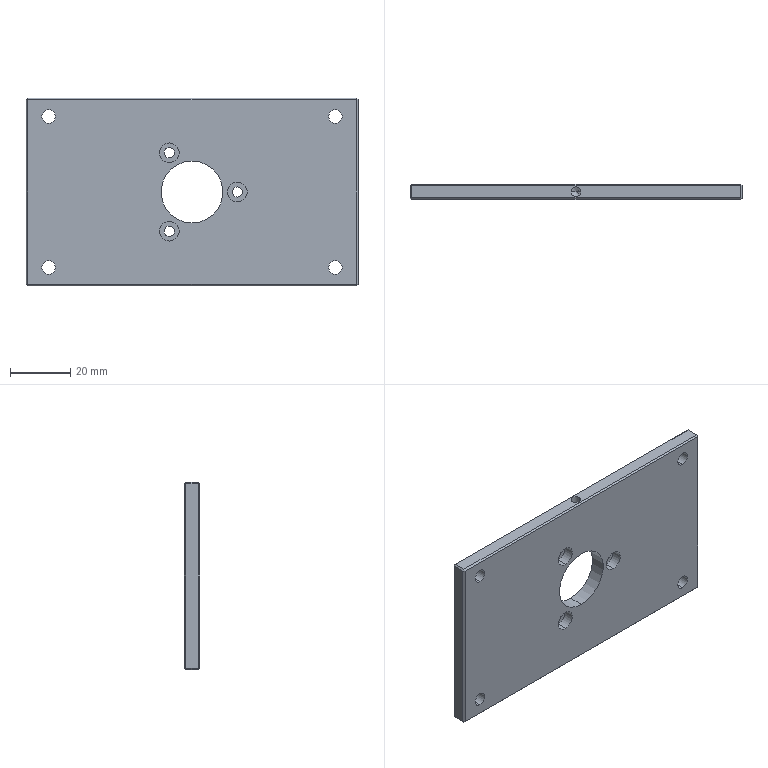Part | STEP file | ND25021-01-JDKM-07-TL | 1 solid | 63 faces | box 110 x 5 x 62 mm | volume 31358 mm3 | plane 29 | cylinder 28 | cone 6 | commonest cylinder face diameters 4.5 x8 3.3 x6 3.4 x6 6.5 x6 20.5 x2